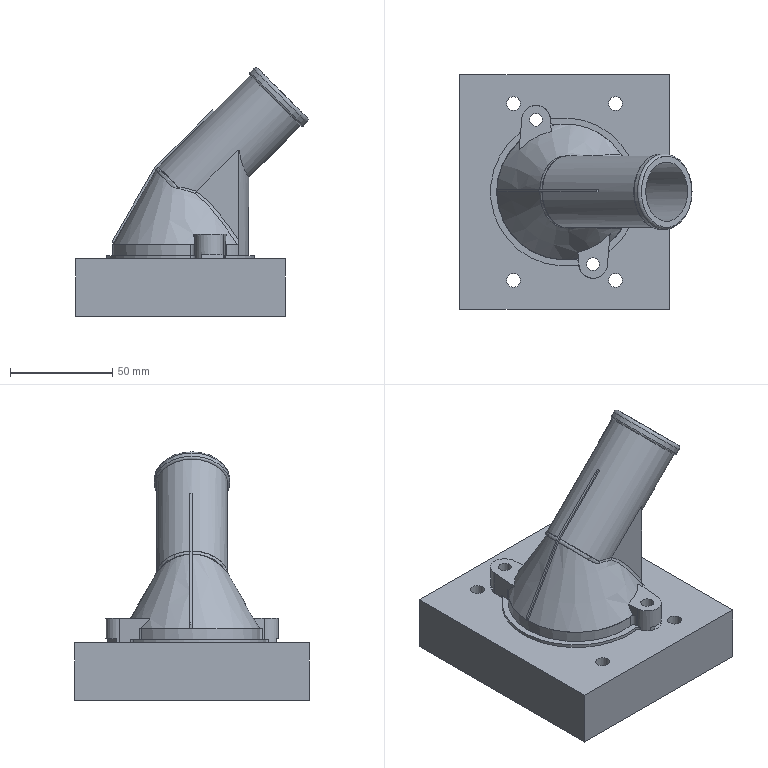Part | 2 solids | 114 faces | box 113.679 x 114.654 x 121.568 mm | volume 343195 mm3 | plane 50 | cylinder 46 | cone 7 | spline 6 | torus 5 | commonest cylinder face diameters 4 x14 6.8 x6 66.5 x5 14 x4 72.5 x4 10 x2